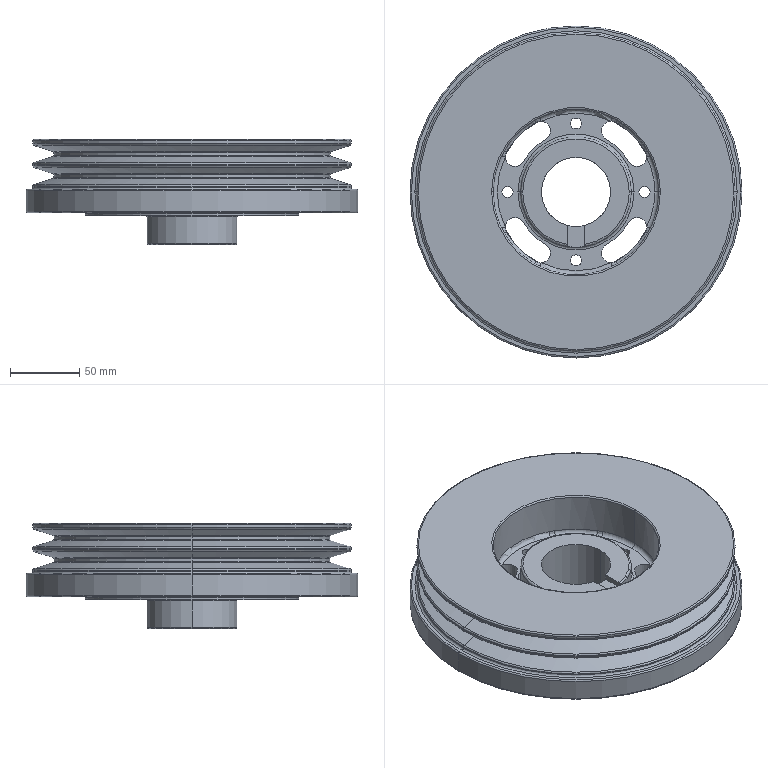Part | SolidWorks | features BaseBody 1 | 1 solid | 146 faces | box 240 x 240 x 76 mm | volume 1699044 mm3 | torus 59 | cylinder 52 | plane 15 | cone 12 | spline 8 | commonest cylinder face diameters 14 x12 8 x8 230 x6 80 x4 88 x4 200 x4